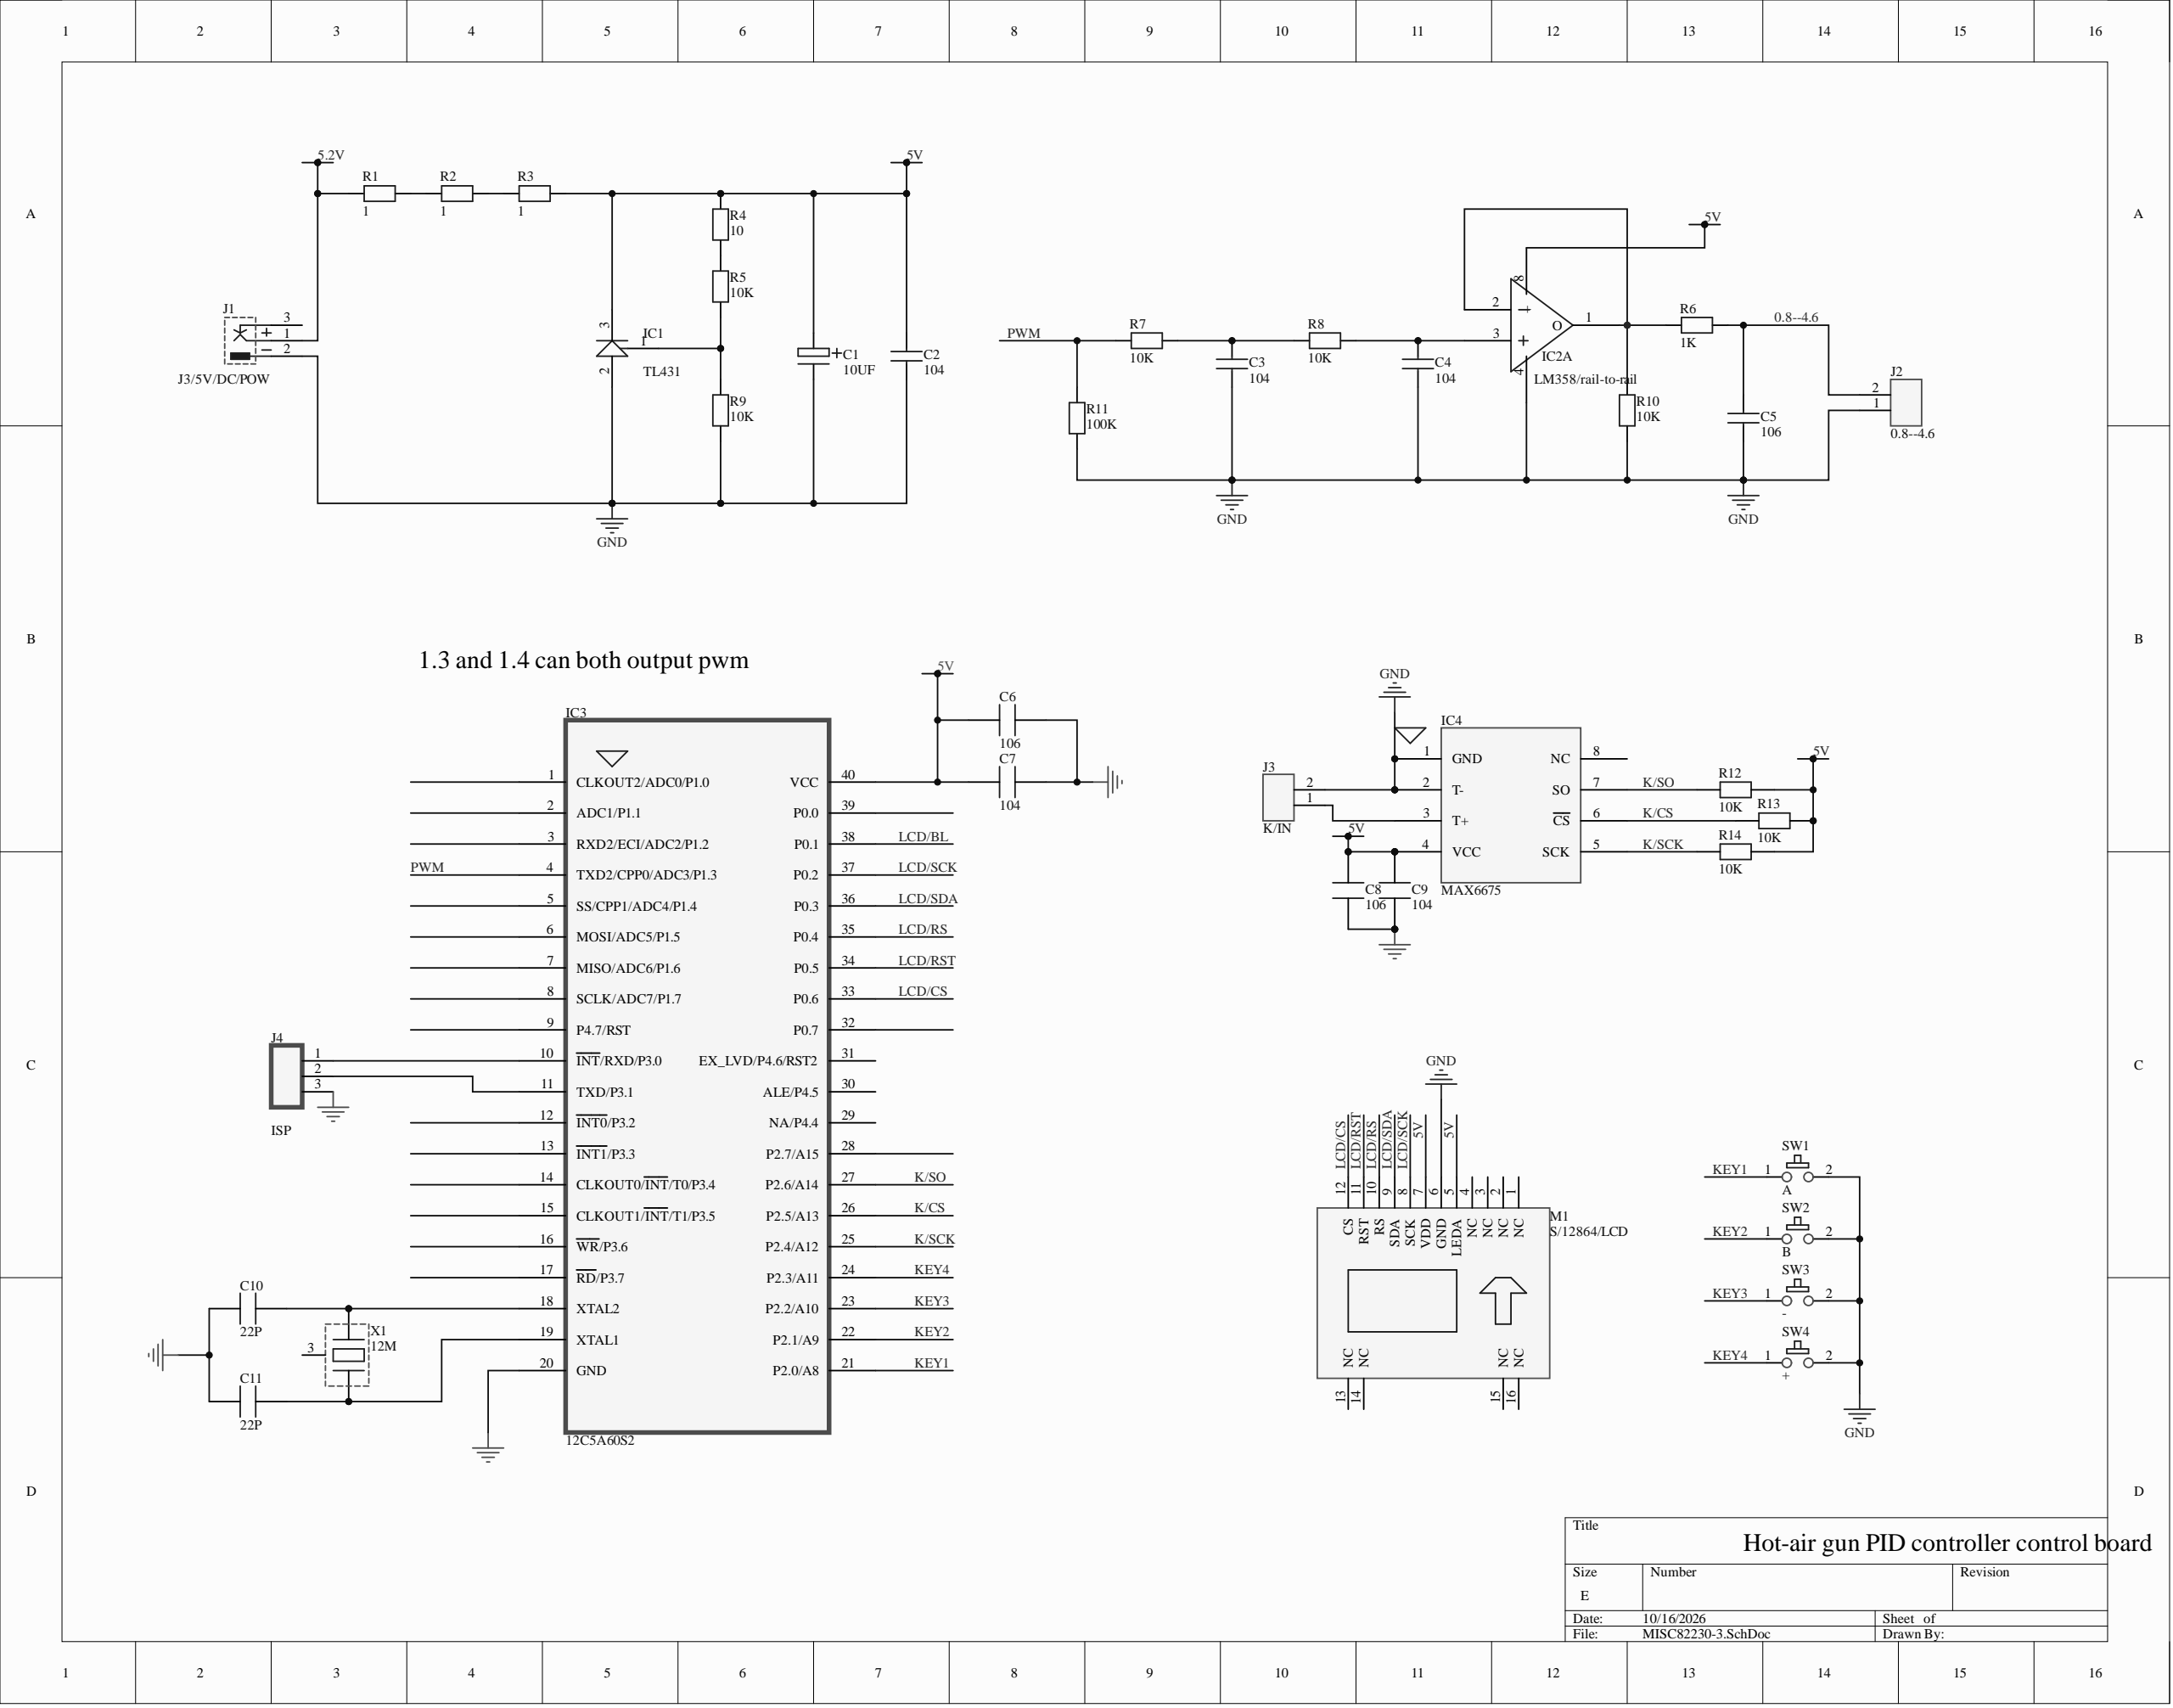Circuit board | Altium Designer | 39 parts | 29 nets
Bill of materials:
Comment,Description,Designator,Footprint,LibRef,Quantity
"10UF","","C1","C10","CE","1"
"104","","C2, C3, C4, C7, C9","0805","C","5"
"106","","C5, C6, C8","0805","C","3"
"22P","","C10, C11","0805","C","2"
"TL431","","IC1","TO92","TL431","1"
"LM358/rail-to-rail","","IC2","SOP8","LM358","1"
"12C5A60S2","","IC3","DIP40","12C5A08AD","1"
"MAX6675","","IC4","SOP8","MAX6675","1"
"J3/5V/DC/POW","","J1","DC/POW","J3/5V/DC/POW","1"
"0.8--4.6","","J2","SIP2/8.5","J2","1"
"K/IN","","J3","SIP2/8.5","J2","1"
"ISP","","J4","SIP3","J3","1"
"S/12864/LCD","","M1","S/12864/LCD","S/12864/LCD","1"
"1","","R1, R2, R3","0805","R","3"
"10","","R4","0805","R","1"
"10K","","R5, R7, R8, R9, R10, R12, R13, R14","0805","R","8"
"1K","","R6","0805","R","1"
"100K","","R11","0805","R","1"
"A","","SW1","BUTTON/B","SW2","1"
"B","","SW2","BUTTON/B","SW2","1"
"-","","SW3","BUTTON/B","SW2","1"
"+","","SW4","BUTTON/B","SW2","1"
"12M","","X1","X","X","1"
Netlist (Protel format):
[
C1
C10
10UF



]
[
C2
0805
104



]
[
C3
0805
104



]
[
C4
0805
104



]
[
C5
0805
106



]
[
C6
0805
106



]
[
C7
0805
104



]
[
C8
0805
106



]
[
C9
0805
104



]
[
C10
0805
22P



]
[
C11
0805
22P



]
[
IC1
TO92
TL431



]
[
IC2
SOP8
LM358/rail-to-rail



]
[
IC3
DIP40
12C5A60S2



]
[
IC4
SOP8
MAX6675



]
[
J1
DC/POW
J3/5V/DC/POW



]
[
J2
SIP2/8.5
0.8--4.6



]
[
J3
SIP2/8.5
K/IN



]
[
J4
SIP3
ISP



]
[
M1
S/12864/LCD
S/12864/LCD



]
[
R1
0805
1



]
[
R2
0805
1



]
[
R3
0805
1



]
[
R4
0805
10



]
[
R5
0805
10K



]
[
R6
0805
1K



]
[
R7
0805
10K



]
[
R8
0805
10K



]
[
R9
0805
10K



]
[
R10
0805
10K



]
[
R11
0805
100K



]
[
R12
0805
10K



]
[
R13
0805
10K



]
[
R14
0805
10K



]
[
SW1
BUTTON/B
A



]
[
SW2
BUTTON/B
B



]
[
SW3
BUTTON/B
-



]
[
SW4
BUTTON/B
+



]
[
X1
X
12M



]
(
PWM
IC3-4
R7-1
R11-2
)
(
NetR4_2
R4-2
R5-1
)
(
NetR2_1
R2-1
R3-2
)
(
NetR1_1
R1-1
R2-2
)
(
NetIC4_3
IC4-3
J3-1
)
(
NetIC3_11
IC3-11
J4-2
)
(
NetIC3_10
IC3-10
J4-1
)
(
NetIC2_1
IC2-1
IC2-2
R6-1
R10-2
)
(
NetIC1_1
IC1-1
R5-2
R9-1
)
(
NetC11_1
C11-1
IC3-19
X1-2
)
(
NetC10_1
C10-1
IC3-18
X1-1
)
(
NetC4_1
C4-1
IC2-3
R8-2
)
(
NetC3_1
C3-1
R7-2
R8-1
)
(
LCD/SDA
IC3-36
M1-9
)
(
LCD/SCK
IC3-37
M1-8
)
(
LCD/RST
IC3-34
M1-11
)
(
LCD/RS
IC3-35
M1-10
)
(
LCD/CS
IC3-33
M1-12
)
(
KEY4
IC3-24
SW4-1
)
(
KEY3
IC3-23
SW3-1
)
(
KEY2
IC3-22
SW2-1
)
(
KEY1
IC3-21
SW1-1
)
(
K/SO
IC3-27
IC4-7
R12-2
)
(
K/SCK
IC3-25
IC4-5
R14-2
)
(
K/CS
IC3-26
IC4-6
R13-2
)
(
GND
C1-2
C2-2
C3-2
C4-2
C5-2
C6-2
C7-2
C8-2
C9-2
C10-2
C11-2
IC1-2
IC2-4
IC3-20
IC4-1
IC4-2
J1-2
J2-1
J3-2
J4-3
M1-6
R9-2
R10-1
R11-1
SW1-2
SW2-2
SW3-2
SW4-2
)
(
5V
C1-1
C2-1
C6-1
C7-1
C8-1
C9-1
IC1-3
IC2-8
IC3-40
IC4-4
M1-5
M1-7
R3-1
R4-1
R12-1
R13-1
R14-1
)
(
5.2V
J1-1
R1-2
)
(
0.8--4.6
C5-1
J2-2
R6-2
)